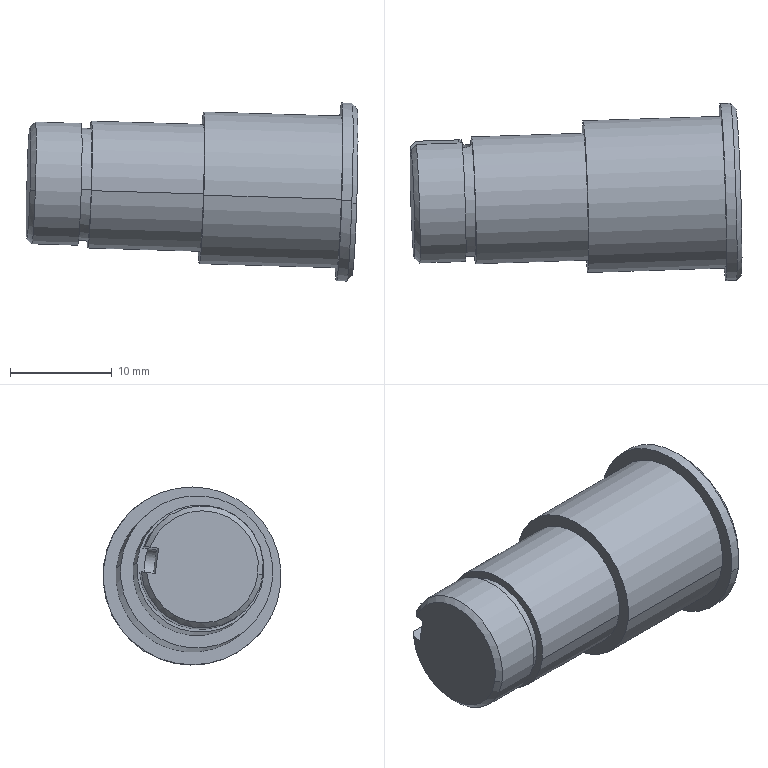Part | STEP file | 2026.6.15-Main Assembly图.sldasm-Part-130 | 1 solid | 24 faces | box 32.571 x 17.473 x 17.472 mm | volume 4708 mm3 | cylinder 11 | plane 9 | cone 4 | commonest cylinder face diameters 11 x3 12.5 x2 14.95 x2 17.45 x2 2.5 x1 12 x1
STEP:
#1=CARTESIAN_POINT('',(-1558.702,1426.585,3693.659));
#2=VERTEX_POINT('',#1);
#3=CARTESIAN_POINT('',(-1558.329,1414.148,3692.46));
#4=VERTEX_POINT('',#3);
#5=CARTESIAN_POINT('',(-1558.516,1420.367,3693.06));
#6=DIRECTION('',(-0.999,-0.03277,0.02917));
#7=DIRECTION('',(-0.02983,0.9949,0.09589));
#8=AXIS2_PLACEMENT_3D('',#5,#6,#7);
#9=CIRCLE('',#8,6.25);
#10=EDGE_CURVE('',#2,#4,#9,.T.);
#11=ORIENTED_EDGE('',*,*,#10,.T.);
#12=CARTESIAN_POINT('',(-1569.319,1413.788,3692.781));
#13=VERTEX_POINT('',#12);
#14=CARTESIAN_POINT('',(-1558.329,1414.148,3692.46));
#15=DIRECTION('',(-0.999,-0.03277,0.02917));
#16=VECTOR('',#15,1000.);
#17=LINE('',#14,#16);
#18=EDGE_CURVE('',#4,#13,#17,.T.);
#19=ORIENTED_EDGE('',*,*,#18,.T.);
#20=CARTESIAN_POINT('',(-1569.692,1426.225,3693.98));
#21=VERTEX_POINT('',#20);
#22=CARTESIAN_POINT('',(-1569.505,1420.006,3693.381));
#23=DIRECTION('',(0.999,0.03277,-0.02917));
#24=DIRECTION('',(-0.02983,0.9949,0.09589));
#25=AXIS2_PLACEMENT_3D('',#22,#23,#24);
#26=CIRCLE('',#25,6.25);
#27=EDGE_CURVE('',#13,#21,#26,.T.);
#28=ORIENTED_EDGE('',*,*,#27,.T.);
#29=CARTESIAN_POINT('',(-1558.702,1426.585,3693.659));
#30=DIRECTION('',(-0.999,-0.03277,0.02917));
#31=VECTOR('',#30,1000.);
#32=LINE('',#29,#31);
#33=EDGE_CURVE('',#2,#21,#32,.T.);
#34=ORIENTED_EDGE('',*,*,#33,.F.);
#35=EDGE_LOOP('',(#11,#19,#28,#34));
#36=FACE_OUTER_BOUND('',#35,.T.);
#37=CARTESIAN_POINT('',(-1558.516,1420.367,3693.06));
#38=DIRECTION('',(-0.999,-0.03277,0.02917));
#39=DIRECTION('',(-0.02983,0.9949,0.09589));
#40=AXIS2_PLACEMENT_3D('',#37,#38,#39);
#41=CYLINDRICAL_SURFACE('',#40,6.25);
#42=ADVANCED_FACE('',(#36),#41,.T.);
#43=CARTESIAN_POINT('',(-1545.252,1428.246,3693.383));
#44=VERTEX_POINT('',#43);
#45=CARTESIAN_POINT('',(-1544.806,1413.372,3691.949));
#46=VERTEX_POINT('',#45);
#47=CARTESIAN_POINT('',(-1545.029,1420.809,3692.666));
#48=DIRECTION('',(-0.999,-0.03277,0.02917));
#49=DIRECTION('',(-0.02983,0.9949,0.09589));
#50=AXIS2_PLACEMENT_3D('',#47,#48,#49);
#51=CIRCLE('',#50,7.475);
#52=EDGE_CURVE('',#44,#46,#51,.T.);
#53=ORIENTED_EDGE('',*,*,#52,.T.);
#54=CARTESIAN_POINT('',(-1558.293,1412.929,3692.343));
#55=VERTEX_POINT('',#54);
#56=CARTESIAN_POINT('',(-1544.806,1413.372,3691.949));
#57=DIRECTION('',(-0.999,-0.03277,0.02917));
#58=VECTOR('',#57,1000.);
#59=LINE('',#56,#58);
#60=EDGE_CURVE('',#46,#55,#59,.T.);
#61=ORIENTED_EDGE('',*,*,#60,.T.);
#62=CARTESIAN_POINT('',(-1558.739,1427.804,3693.776));
#63=VERTEX_POINT('',#62);
#64=CARTESIAN_POINT('',(-1558.516,1420.367,3693.06));
#65=DIRECTION('',(0.999,0.03277,-0.02917));
#66=DIRECTION('',(-0.02983,0.9949,0.09589));
#67=AXIS2_PLACEMENT_3D('',#64,#65,#66);
#68=CIRCLE('',#67,7.475);
#69=EDGE_CURVE('',#55,#63,#68,.T.);
#70=ORIENTED_EDGE('',*,*,#69,.T.);
#71=CARTESIAN_POINT('',(-1545.252,1428.246,3693.383));
#72=DIRECTION('',(-0.999,-0.03277,0.02917));
#73=VECTOR('',#72,1000.);
#74=LINE('',#71,#73);
#75=EDGE_CURVE('',#44,#63,#74,.T.);
#76=ORIENTED_EDGE('',*,*,#75,.F.);
#77=EDGE_LOOP('',(#53,#61,#70,#76));
#78=FACE_OUTER_BOUND('',#77,.T.);
#79=CARTESIAN_POINT('',(-1545.029,1420.809,3692.666));
#80=DIRECTION('',(-0.999,-0.03277,0.02917));
#81=DIRECTION('',(-0.02983,0.9949,0.09589));
#82=AXIS2_PLACEMENT_3D('',#79,#80,#81);
#83=CYLINDRICAL_SURFACE('',#82,7.475);
#84=ADVANCED_FACE('',(#78),#83,.T.);
#85=CARTESIAN_POINT('',(-1543.294,1412.706,3691.557));
#86=VERTEX_POINT('',#85);
#87=CARTESIAN_POINT('',(-1543.767,1429.01,3693.687));
#88=VERTEX_POINT('',#87);
#89=CARTESIAN_POINT('',(-1543.53,1420.858,3692.622));
#90=DIRECTION('',(0.999,0.03277,-0.02917));
#91=DIRECTION('',(0.02873,-0.9912,-0.1295));
#92=AXIS2_PLACEMENT_3D('',#89,#90,#91);
#93=CIRCLE('',#92,8.225);
#94=EDGE_CURVE('',#86,#88,#93,.T.);
#95=ORIENTED_EDGE('',*,*,#94,.F.);
#96=CARTESIAN_POINT('',(-1543.779,1412.194,3691.507));
#97=VERTEX_POINT('',#96);
#98=CARTESIAN_POINT('',(-1543.779,1412.194,3691.507));
#99=DIRECTION('',(-0.6861,-0.724,-0.07092));
#100=VECTOR('',#99,1000.);
#101=LINE('',#98,#100);
#102=EDGE_CURVE('',#86,#97,#101,.T.);
#103=ORIENTED_EDGE('',*,*,#102,.T.);
#104=CARTESIAN_POINT('',(-1544.29,1429.523,3693.473));
#105=VERTEX_POINT('',#104);
#106=CARTESIAN_POINT('',(-1544.03,1420.842,3692.637));
#107=DIRECTION('',(-0.999,-0.03277,0.02917));
#108=DIRECTION('',(0.02873,-0.9912,-0.1295));
#109=AXIS2_PLACEMENT_3D('',#106,#107,#108);
#110=CIRCLE('',#109,8.725);
#111=EDGE_CURVE('',#105,#97,#110,.T.);
#112=ORIENTED_EDGE('',*,*,#111,.F.);
#113=CARTESIAN_POINT('',(-1544.281,1429.49,3693.766));
#114=VERTEX_POINT('',#113);
#115=CARTESIAN_POINT('',(-1544.03,1420.842,3692.637));
#116=DIRECTION('',(-0.999,-0.03277,0.02917));
#117=DIRECTION('',(0.02873,-0.9912,-0.1295));
#118=AXIS2_PLACEMENT_3D('',#115,#116,#117);
#119=CIRCLE('',#118,8.725);
#120=EDGE_CURVE('',#114,#105,#119,.T.);
#121=ORIENTED_EDGE('',*,*,#120,.F.);
#122=CARTESIAN_POINT('',(-1544.281,1429.49,3693.766));
#123=DIRECTION('',(-0.7267,0.6777,0.1122));
#124=VECTOR('',#123,1000.);
#125=LINE('',#122,#124);
#126=EDGE_CURVE('',#88,#114,#125,.T.);
#127=ORIENTED_EDGE('',*,*,#126,.F.);
#128=EDGE_LOOP('',(#95,#103,#112,#121,#127));
#129=FACE_OUTER_BOUND('',#128,.T.);
#130=CARTESIAN_POINT('',(-1544.03,1420.842,3692.637));
#131=DIRECTION('',(-0.999,-0.03277,0.02917));
#132=DIRECTION('',(-0.02873,0.9912,0.1295));
#133=AXIS2_PLACEMENT_3D('',#130,#131,#132);
#134=CONICAL_SURFACE('',#133,8.725,0.7854);
#135=ADVANCED_FACE('',(#129),#134,.T.);
#136=ORIENTED_EDGE('',*,*,#111,.T.);
#137=CARTESIAN_POINT('',(-1543.77,1412.161,3691.8));
#138=VERTEX_POINT('',#137);
#139=CARTESIAN_POINT('',(-1544.03,1420.842,3692.637));
#140=DIRECTION('',(-0.999,-0.03277,0.02917));
#141=DIRECTION('',(0.02873,-0.9912,-0.1295));
#142=AXIS2_PLACEMENT_3D('',#139,#140,#141);
#143=CIRCLE('',#142,8.725);
#144=EDGE_CURVE('',#97,#138,#143,.T.);
#145=ORIENTED_EDGE('',*,*,#144,.T.);
#146=CARTESIAN_POINT('',(-1544.769,1412.128,3691.829));
#147=VERTEX_POINT('',#146);
#148=CARTESIAN_POINT('',(-1543.27,1412.177,3691.785));
#149=DIRECTION('',(-0.999,-0.03277,0.02917));
#150=VECTOR('',#149,1000.);
#151=LINE('',#148,#150);
#152=EDGE_CURVE('',#138,#147,#151,.T.);
#153=ORIENTED_EDGE('',*,*,#152,.T.);
#154=CARTESIAN_POINT('',(-1545.289,1429.49,3693.502));
#155=VERTEX_POINT('',#154);
#156=CARTESIAN_POINT('',(-1545.029,1420.809,3692.666));
#157=DIRECTION('',(0.999,0.03277,-0.02917));
#158=DIRECTION('',(-0.02983,0.9949,0.09589));
#159=AXIS2_PLACEMENT_3D('',#156,#157,#158);
#160=CIRCLE('',#159,8.725);
#161=EDGE_CURVE('',#147,#155,#160,.T.);
#162=ORIENTED_EDGE('',*,*,#161,.T.);
#163=CARTESIAN_POINT('',(-1543.791,1429.539,3693.459));
#164=DIRECTION('',(-0.999,-0.03277,0.02917));
#165=VECTOR('',#164,1000.);
#166=LINE('',#163,#165);
#167=EDGE_CURVE('',#105,#155,#166,.T.);
#168=ORIENTED_EDGE('',*,*,#167,.F.);
#169=EDGE_LOOP('',(#136,#145,#153,#162,#168));
#170=FACE_OUTER_BOUND('',#169,.T.);
#171=CARTESIAN_POINT('',(-1543.53,1420.858,3692.622));
#172=DIRECTION('',(-0.999,-0.03277,0.02917));
#173=DIRECTION('',(-0.02983,0.9949,0.09589));
#174=AXIS2_PLACEMENT_3D('',#171,#172,#173);
#175=CYLINDRICAL_SURFACE('',#174,8.725);
#176=ADVANCED_FACE('',(#170),#175,.T.);
#177=CARTESIAN_POINT('',(-1575.342,1414.358,3692.843));
#178=VERTEX_POINT('',#177);
#179=CARTESIAN_POINT('',(-1575.612,1424.958,3695.488));
#180=VERTEX_POINT('',#179);
#181=CARTESIAN_POINT('',(-1575.5,1419.809,3693.556));
#182=DIRECTION('',(-0.999,-0.03277,0.02917));
#183=DIRECTION('',(-0.02873,0.9912,0.1295));
#184=AXIS2_PLACEMENT_3D('',#181,#182,#183);
#185=CIRCLE('',#184,5.5);
#186=EDGE_CURVE('',#178,#180,#185,.T.);
#187=ORIENTED_EDGE('',*,*,#186,.F.);
#188=CARTESIAN_POINT('',(-1574.828,1413.879,3692.764));
#189=VERTEX_POINT('',#188);
#190=CARTESIAN_POINT('',(-1574.828,1413.879,3692.764));
#191=DIRECTION('',(0.7267,-0.6777,-0.1122));
#192=VECTOR('',#191,1000.);
#193=LINE('',#190,#192);
#194=EDGE_CURVE('',#178,#189,#193,.T.);
#195=ORIENTED_EDGE('',*,*,#194,.T.);
#196=CARTESIAN_POINT('',(-1575.127,1425.482,3695.54));
#197=VERTEX_POINT('',#196);
#198=CARTESIAN_POINT('',(-1575.,1419.826,3693.541));
#199=DIRECTION('',(0.999,0.03277,-0.02917));
#200=DIRECTION('',(-0.02873,0.9912,0.1295));
#201=AXIS2_PLACEMENT_3D('',#198,#199,#200);
#202=CIRCLE('',#201,6.);
#203=EDGE_CURVE('',#197,#189,#202,.T.);
#204=ORIENTED_EDGE('',*,*,#203,.F.);
#205=CARTESIAN_POINT('',(-1575.127,1425.482,3695.54));
#206=CARTESIAN_POINT('',(-1575.289,1425.307,3695.523));
#207=CARTESIAN_POINT('',(-1575.451,1425.132,3695.505));
#208=CARTESIAN_POINT('',(-1575.612,1424.958,3695.488));
#209=B_SPLINE_CURVE_WITH_KNOTS('',3,(#205,#206,#207,#208),.UNSPECIFIED.,.F.,.F.,(4,4),(0.002943,0.003659),.UNSPECIFIED.);
#210=EDGE_CURVE('',#197,#180,#209,.T.);
#211=ORIENTED_EDGE('',*,*,#210,.T.);
#212=EDGE_LOOP('',(#187,#195,#204,#211));
#213=FACE_OUTER_BOUND('',#212,.T.);
#214=CARTESIAN_POINT('',(-1575.,1419.826,3693.541));
#215=DIRECTION('',(0.999,0.03277,-0.02917));
#216=DIRECTION('',(0.02873,-0.9912,-0.1295));
#217=AXIS2_PLACEMENT_3D('',#214,#215,#216);
#218=CONICAL_SURFACE('',#217,6.,0.7854);
#219=ADVANCED_FACE('',(#213),#218,.T.);
#220=CARTESIAN_POINT('',(-1569.669,1425.478,3693.908));
#221=VERTEX_POINT('',#220);
#222=CARTESIAN_POINT('',(-1569.341,1414.534,3692.853));
#223=VERTEX_POINT('',#222);
#224=CARTESIAN_POINT('',(-1569.505,1420.006,3693.381));
#225=DIRECTION('',(-0.999,-0.03277,0.02917));
#226=DIRECTION('',(-0.02983,0.9949,0.09589));
#227=AXIS2_PLACEMENT_3D('',#224,#225,#226);
#228=CIRCLE('',#227,5.5);
#229=EDGE_CURVE('',#221,#223,#228,.T.);
#230=ORIENTED_EDGE('',*,*,#229,.T.);
#231=CARTESIAN_POINT('',(-1570.34,1414.501,3692.882));
#232=VERTEX_POINT('',#231);
#233=CARTESIAN_POINT('',(-1569.341,1414.534,3692.853));
#234=DIRECTION('',(-0.999,-0.03277,0.02917));
#235=VECTOR('',#234,1000.);
#236=LINE('',#233,#235);
#237=EDGE_CURVE('',#223,#232,#236,.T.);
#238=ORIENTED_EDGE('',*,*,#237,.T.);
#239=CARTESIAN_POINT('',(-1570.699,1425.445,3692.89));
#240=VERTEX_POINT('',#239);
#241=CARTESIAN_POINT('',(-1570.504,1419.973,3693.41));
#242=DIRECTION('',(0.999,0.03277,-0.02917));
#243=DIRECTION('',(-0.02983,0.9949,0.09589));
#244=AXIS2_PLACEMENT_3D('',#241,#242,#243);
#245=CIRCLE('',#244,5.5);
#246=EDGE_CURVE('',#232,#240,#245,.T.);
#247=ORIENTED_EDGE('',*,*,#246,.T.);
#248=CARTESIAN_POINT('',(-1569.683,1425.478,3693.908));
#249=VERTEX_POINT('',#248);
#250=CARTESIAN_POINT('',(-1570.699,1425.445,3692.89));
#251=CARTESIAN_POINT('',(-1570.572,1425.452,3692.913));
#252=CARTESIAN_POINT('',(-1570.452,1425.46,3692.954));
#253=CARTESIAN_POINT('',(-1570.226,1425.476,3693.074));
#254=CARTESIAN_POINT('',(-1570.123,1425.484,3693.15));
#255=CARTESIAN_POINT('',(-1569.853,1425.501,3693.422));
#256=CARTESIAN_POINT('',(-1569.729,1425.5,3693.66));
#257=CARTESIAN_POINT('',(-1569.683,1425.478,3693.908));
#258=B_SPLINE_CURVE_WITH_KNOTS('',3,(#250,#251,#252,#253,#254,#255,#256,#257),.UNSPECIFIED.,.F.,.F.,(4,2,2,4),(0.,0.0003812,0.0007624,0.001525),.UNSPECIFIED.);
#259=EDGE_CURVE('',#240,#249,#258,.T.);
#260=ORIENTED_EDGE('',*,*,#259,.T.);
#261=CARTESIAN_POINT('',(-1569.669,1425.478,3693.908));
#262=DIRECTION('',(-0.999,-0.03277,0.02917));
#263=VECTOR('',#262,1000.);
#264=LINE('',#261,#263);
#265=EDGE_CURVE('',#221,#249,#264,.T.);
#266=ORIENTED_EDGE('',*,*,#265,.F.);
#267=EDGE_LOOP('',(#230,#238,#247,#260,#266));
#268=FACE_OUTER_BOUND('',#267,.T.);
#269=CARTESIAN_POINT('',(-1569.505,1420.006,3693.381));
#270=DIRECTION('',(-0.999,-0.03277,0.02917));
#271=DIRECTION('',(-0.02983,0.9949,0.09589));
#272=AXIS2_PLACEMENT_3D('',#269,#270,#271);
#273=CYLINDRICAL_SURFACE('',#272,5.5);
#274=ADVANCED_FACE('',(#268),#273,.T.);
#275=CARTESIAN_POINT('',(-1569.663,1425.458,3694.093));
#276=VERTEX_POINT('',#275);
#277=CARTESIAN_POINT('',(-1569.505,1420.006,3693.381));
#278=DIRECTION('',(-0.999,-0.03277,0.02917));
#279=DIRECTION('',(-0.02983,0.9949,0.09589));
#280=AXIS2_PLACEMENT_3D('',#277,#278,#279);
#281=CIRCLE('',#280,5.5);
#282=EDGE_CURVE('',#276,#221,#281,.T.);
#283=ORIENTED_EDGE('',*,*,#282,.T.);
#284=ORIENTED_EDGE('',*,*,#265,.T.);
#285=CARTESIAN_POINT('',(-1569.683,1425.478,3693.908));
#286=CARTESIAN_POINT('',(-1569.672,1425.472,3693.969));
#287=CARTESIAN_POINT('',(-1569.665,1425.466,3694.03));
#288=CARTESIAN_POINT('',(-1569.663,1425.458,3694.093));
#289=B_SPLINE_CURVE_WITH_KNOTS('',3,(#285,#286,#287,#288),.UNSPECIFIED.,.F.,.F.,(4,4),(0.001525,0.001711),.UNSPECIFIED.);
#290=EDGE_CURVE('',#249,#276,#289,.T.);
#291=ORIENTED_EDGE('',*,*,#290,.T.);
#292=EDGE_LOOP('',(#283,#284,#291));
#293=FACE_OUTER_BOUND('',#292,.T.);
#294=CARTESIAN_POINT('',(-1569.505,1420.006,3693.381));
#295=DIRECTION('',(-0.999,-0.03277,0.02917));
#296=DIRECTION('',(-0.02983,0.9949,0.09589));
#297=AXIS2_PLACEMENT_3D('',#294,#295,#296);
#298=CYLINDRICAL_SURFACE('',#297,5.5);
#299=ADVANCED_FACE('',(#293),#298,.T.);
#300=ORIENTED_EDGE('',*,*,#237,.F.);
#301=CARTESIAN_POINT('',(-1569.505,1420.006,3693.381));
#302=DIRECTION('',(-0.999,-0.03277,0.02917));
#303=DIRECTION('',(-0.02983,0.9949,0.09589));
#304=AXIS2_PLACEMENT_3D('',#301,#302,#303);
#305=CIRCLE('',#304,5.5);
#306=EDGE_CURVE('',#223,#276,#305,.T.);
#307=ORIENTED_EDGE('',*,*,#306,.T.);
#308=CARTESIAN_POINT('',(-1570.618,1425.13,3695.318));
#309=VERTEX_POINT('',#308);
#310=CARTESIAN_POINT('',(-1569.663,1425.458,3694.093));
#311=CARTESIAN_POINT('',(-1569.659,1425.439,3694.236));
#312=CARTESIAN_POINT('',(-1569.678,1425.414,3694.376));
#313=CARTESIAN_POINT('',(-1569.766,1425.356,3694.645));
#314=CARTESIAN_POINT('',(-1569.831,1425.323,3694.768));
#315=CARTESIAN_POINT('',(-1570.004,1425.257,3694.989));
#316=CARTESIAN_POINT('',(-1570.109,1425.224,3695.082));
#317=CARTESIAN_POINT('',(-1570.348,1425.168,3695.232));
#318=CARTESIAN_POINT('',(-1570.478,1425.145,3695.286));
#319=CARTESIAN_POINT('',(-1570.618,1425.13,3695.318));
#320=B_SPLINE_CURVE_WITH_KNOTS('',3,(#310,#311,#312,#313,#314,#315,#316,#317,#318,#319),.UNSPECIFIED.,.F.,.F.,(4,2,2,2,4),(0.,0.0004277,0.0008554,0.001283,0.001711),.UNSPECIFIED.);
#321=EDGE_CURVE('',#276,#309,#320,.T.);
#322=ORIENTED_EDGE('',*,*,#321,.T.);
#323=CARTESIAN_POINT('',(-1570.504,1419.973,3693.41));
#324=DIRECTION('',(0.999,0.03277,-0.02917));
#325=DIRECTION('',(-0.02983,0.9949,0.09589));
#326=AXIS2_PLACEMENT_3D('',#323,#324,#325);
#327=CIRCLE('',#326,5.5);
#328=EDGE_CURVE('',#309,#232,#327,.T.);
#329=ORIENTED_EDGE('',*,*,#328,.T.);
#330=EDGE_LOOP('',(#300,#307,#322,#329));
#331=FACE_OUTER_BOUND('',#330,.T.);
#332=CARTESIAN_POINT('',(-1569.505,1420.006,3693.381));
#333=DIRECTION('',(-0.999,-0.03277,0.02917));
#334=DIRECTION('',(-0.02983,0.9949,0.09589));
#335=AXIS2_PLACEMENT_3D('',#332,#333,#334);
#336=CYLINDRICAL_SURFACE('',#335,5.5);
#337=ADVANCED_FACE('',(#331),#336,.T.);
#338=ORIENTED_EDGE('',*,*,#328,.F.);
#339=CARTESIAN_POINT('',(-1570.633,1425.638,3695.384));
#340=VERTEX_POINT('',#339);
#341=CARTESIAN_POINT('',(-1570.618,1425.13,3695.318));
#342=DIRECTION('',(-0.02873,0.9912,0.1295));
#343=VECTOR('',#342,1000.);
#344=LINE('',#341,#343);
#345=EDGE_CURVE('',#309,#340,#344,.T.);
#346=ORIENTED_EDGE('',*,*,#345,.T.);
#347=CARTESIAN_POINT('',(-1570.714,1425.953,3692.956));
#348=VERTEX_POINT('',#347);
#349=CARTESIAN_POINT('',(-1570.504,1419.973,3693.41));
#350=DIRECTION('',(-0.999,-0.03277,0.02917));
#351=DIRECTION('',(-0.02983,0.9949,0.09589));
#352=AXIS2_PLACEMENT_3D('',#349,#350,#351);
#353=CIRCLE('',#352,6.);
#354=EDGE_CURVE('',#348,#340,#353,.T.);
#355=ORIENTED_EDGE('',*,*,#354,.F.);
#356=CARTESIAN_POINT('',(-1570.714,1425.953,3692.956));
#357=DIRECTION('',(0.02873,-0.9912,-0.1295));
#358=VECTOR('',#357,1000.);
#359=LINE('',#356,#358);
#360=EDGE_CURVE('',#348,#240,#359,.T.);
#361=ORIENTED_EDGE('',*,*,#360,.T.);
#362=ORIENTED_EDGE('',*,*,#246,.F.);
#363=EDGE_LOOP('',(#338,#346,#355,#361,#362));
#364=FACE_OUTER_BOUND('',#363,.T.);
#365=CARTESIAN_POINT('',(-1570.504,1419.973,3693.41));
#366=DIRECTION('',(0.999,0.03277,-0.02917));
#367=DIRECTION('',(0.02873,-0.9912,-0.1295));
#368=AXIS2_PLACEMENT_3D('',#365,#366,#367);
#369=PLANE('',#368);
#370=ADVANCED_FACE('',(#364),#369,.T.);
#371=ORIENTED_EDGE('',*,*,#354,.T.);
#372=CARTESIAN_POINT('',(-1570.881,1425.621,3695.416));
#373=VERTEX_POINT('',#372);
#374=CARTESIAN_POINT('',(-1570.633,1425.638,3695.384));
#375=CARTESIAN_POINT('',(-1570.714,1425.629,3695.403));
#376=CARTESIAN_POINT('',(-1570.797,1425.624,3695.413));
#377=CARTESIAN_POINT('',(-1570.881,1425.621,3695.416));
#378=B_SPLINE_CURVE_WITH_KNOTS('',3,(#374,#375,#376,#377),.UNSPECIFIED.,.F.,.F.,(4,4),(0.,0.0002513),.UNSPECIFIED.);
#379=EDGE_CURVE('',#340,#373,#378,.T.);
#380=ORIENTED_EDGE('',*,*,#379,.T.);
#381=CARTESIAN_POINT('',(-1570.632,1425.629,3695.408));
#382=DIRECTION('',(-0.999,-0.03277,0.02917));
#383=VECTOR('',#382,1000.);
#384=LINE('',#381,#383);
#385=EDGE_CURVE('',#373,#197,#384,.T.);
#386=ORIENTED_EDGE('',*,*,#385,.T.);
#387=ORIENTED_EDGE('',*,*,#203,.T.);
#388=CARTESIAN_POINT('',(-1575.21,1425.803,3693.062));
#389=VERTEX_POINT('',#388);
#390=CARTESIAN_POINT('',(-1575.,1419.826,3693.541));
#391=DIRECTION('',(0.999,0.03277,-0.02917));
#392=DIRECTION('',(-0.02873,0.9912,0.1295));
#393=AXIS2_PLACEMENT_3D('',#390,#391,#392);
#394=CIRCLE('',#393,6.);
#395=EDGE_CURVE('',#189,#389,#394,.T.);
#396=ORIENTED_EDGE('',*,*,#395,.T.);
#397=CARTESIAN_POINT('',(-1570.964,1425.942,3692.938));
#398=VERTEX_POINT('',#397);
#399=CARTESIAN_POINT('',(-1570.714,1425.95,3692.931));
#400=DIRECTION('',(-0.999,-0.03277,0.02917));
#401=VECTOR('',#400,1000.);
#402=LINE('',#399,#401);
#403=EDGE_CURVE('',#398,#389,#402,.T.);
#404=ORIENTED_EDGE('',*,*,#403,.F.);
#405=CARTESIAN_POINT('',(-1570.964,1425.942,3692.938));
#406=CARTESIAN_POINT('',(-1570.88,1425.945,3692.935));
#407=CARTESIAN_POINT('',(-1570.797,1425.948,3692.942));
#408=CARTESIAN_POINT('',(-1570.714,1425.953,3692.956));
#409=B_SPLINE_CURVE_WITH_KNOTS('',3,(#405,#406,#407,#408),.UNSPECIFIED.,.F.,.F.,(4,4),(0.,0.0002513),.UNSPECIFIED.);
#410=EDGE_CURVE('',#398,#348,#409,.T.);
#411=ORIENTED_EDGE('',*,*,#410,.T.);
#412=EDGE_LOOP('',(#371,#380,#386,#387,#396,#404,#411));
#413=FACE_OUTER_BOUND('',#412,.T.);
#414=CARTESIAN_POINT('',(-1570.504,1419.973,3693.41));
#415=DIRECTION('',(-0.999,-0.03277,0.02917));
#416=DIRECTION('',(-0.02983,0.9949,0.09589));
#417=AXIS2_PLACEMENT_3D('',#414,#415,#416);
#418=CYLINDRICAL_SURFACE('',#417,6.);
#419=ADVANCED_FACE('',(#413),#418,.T.);
#420=ORIENTED_EDGE('',*,*,#194,.F.);
#421=CARTESIAN_POINT('',(-1575.695,1425.279,3693.01));
#422=VERTEX_POINT('',#421);
#423=CARTESIAN_POINT('',(-1575.5,1419.809,3693.556));
#424=DIRECTION('',(-0.999,-0.03277,0.02917));
#425=DIRECTION('',(-0.02873,0.9912,0.1295));
#426=AXIS2_PLACEMENT_3D('',#423,#424,#425);
#427=CIRCLE('',#426,5.5);
#428=EDGE_CURVE('',#422,#178,#427,.T.);
#429=ORIENTED_EDGE('',*,*,#428,.F.);
#430=CARTESIAN_POINT('',(-1575.21,1425.803,3693.062));
#431=CARTESIAN_POINT('',(-1575.372,1425.628,3693.045));
#432=CARTESIAN_POINT('',(-1575.534,1425.454,3693.027));
#433=CARTESIAN_POINT('',(-1575.695,1425.279,3693.01));
#434=B_SPLINE_CURVE_WITH_KNOTS('',3,(#430,#431,#432,#433),.UNSPECIFIED.,.F.,.F.,(4,4),(0.002943,0.003659),.UNSPECIFIED.);
#435=EDGE_CURVE('',#389,#422,#434,.T.);
#436=ORIENTED_EDGE('',*,*,#435,.F.);
#437=ORIENTED_EDGE('',*,*,#395,.F.);
#438=EDGE_LOOP('',(#420,#429,#436,#437));
#439=FACE_OUTER_BOUND('',#438,.T.);
#440=CARTESIAN_POINT('',(-1575.,1419.826,3693.541));
#441=DIRECTION('',(0.999,0.03277,-0.02917));
#442=DIRECTION('',(0.02873,-0.9912,-0.1295));
#443=AXIS2_PLACEMENT_3D('',#440,#441,#442);
#444=CONICAL_SURFACE('',#443,6.,0.7854);
#445=ADVANCED_FACE('',(#439),#444,.T.);
#446=ORIENTED_EDGE('',*,*,#52,.F.);
#447=CARTESIAN_POINT('',(-1545.029,1420.809,3692.666));
#448=DIRECTION('',(-0.999,-0.03277,0.02917));
#449=DIRECTION('',(-0.02983,0.9949,0.09589));
#450=AXIS2_PLACEMENT_3D('',#447,#448,#449);
#451=CIRCLE('',#450,7.475);
#452=EDGE_CURVE('',#46,#44,#451,.T.);
#453=ORIENTED_EDGE('',*,*,#452,.F.);
#454=EDGE_LOOP('',(#446,#453));
#455=FACE_BOUND('',#454,.T.);
#456=CARTESIAN_POINT('',(-1545.029,1420.809,3692.666));
#457=DIRECTION('',(0.999,0.03277,-0.02917));
#458=DIRECTION('',(-0.02983,0.9949,0.09589));
#459=AXIS2_PLACEMENT_3D('',#456,#457,#458);
#460=CIRCLE('',#459,8.725);
#461=EDGE_CURVE('',#155,#147,#460,.T.);
#462=ORIENTED_EDGE('',*,*,#461,.F.);
#463=ORIENTED_EDGE('',*,*,#161,.F.);
#464=EDGE_LOOP('',(#462,#463));
#465=FACE_OUTER_BOUND('',#464,.T.);
#466=CARTESIAN_POINT('',(-1545.029,1420.809,3692.666));
#467=DIRECTION('',(-0.999,-0.03277,0.02917));
#468=DIRECTION('',(-0.02873,0.9912,0.1295));
#469=AXIS2_PLACEMENT_3D('',#466,#467,#468);
#470=PLANE('',#469);
#471=ADVANCED_FACE('',(#455,#465),#470,.T.);
#472=CARTESIAN_POINT('',(-1543.53,1420.858,3692.622));
#473=DIRECTION('',(0.999,0.03277,-0.02917));
#474=DIRECTION('',(0.02873,-0.9912,-0.1295));
#475=AXIS2_PLACEMENT_3D('',#472,#473,#474);
#476=CIRCLE('',#475,8.225);
#477=EDGE_CURVE('',#88,#86,#476,.T.);
#478=ORIENTED_EDGE('',*,*,#477,.T.);
#479=ORIENTED_EDGE('',*,*,#94,.T.);
#480=EDGE_LOOP('',(#478,#479));
#481=FACE_OUTER_BOUND('',#480,.T.);
#482=CARTESIAN_POINT('',(-1543.53,1420.858,3692.622));
#483=DIRECTION('',(0.999,0.03277,-0.02917));
#484=DIRECTION('',(0.02873,-0.9912,-0.1295));
#485=AXIS2_PLACEMENT_3D('',#482,#483,#484);
#486=PLANE('',#485);
#487=ADVANCED_FACE('',(#481),#486,.T.);
#488=ORIENTED_EDGE('',*,*,#152,.F.);
#489=CARTESIAN_POINT('',(-1544.03,1420.842,3692.637));
#490=DIRECTION('',(-0.999,-0.03277,0.02917));
#491=DIRECTION('',(0.02873,-0.9912,-0.1295));
#492=AXIS2_PLACEMENT_3D('',#489,#490,#491);
#493=CIRCLE('',#492,8.725);
#494=EDGE_CURVE('',#138,#114,#493,.T.);
#495=ORIENTED_EDGE('',*,*,#494,.T.);
#496=ORIENTED_EDGE('',*,*,#120,.T.);
#497=ORIENTED_EDGE('',*,*,#167,.T.);
#498=ORIENTED_EDGE('',*,*,#461,.T.);
#499=EDGE_LOOP('',(#488,#495,#496,#497,#498));
#500=FACE_OUTER_BOUND('',#499,.T.);
#501=CARTESIAN_POINT('',(-1543.53,1420.858,3692.622));
#502=DIRECTION('',(-0.999,-0.03277,0.02917));
#503=DIRECTION('',(-0.02983,0.9949,0.09589));
#504=AXIS2_PLACEMENT_3D('',#501,#502,#503);
#505=CYLINDRICAL_SURFACE('',#504,8.725);
#506=ADVANCED_FACE('',(#500),#505,.T.);
#507=ORIENTED_EDGE('',*,*,#102,.F.);
#508=ORIENTED_EDGE('',*,*,#477,.F.);
#509=ORIENTED_EDGE('',*,*,#126,.T.);
#510=ORIENTED_EDGE('',*,*,#494,.F.);
#511=ORIENTED_EDGE('',*,*,#144,.F.);
#512=EDGE_LOOP('',(#507,#508,#509,#510,#511));
#513=FACE_OUTER_BOUND('',#512,.T.);
#514=CARTESIAN_POINT('',(-1544.03,1420.842,3692.637));
#515=DIRECTION('',(-0.999,-0.03277,0.02917));
#516=DIRECTION('',(-0.02873,0.9912,0.1295));
#517=AXIS2_PLACEMENT_3D('',#514,#515,#516);
#518=CONICAL_SURFACE('',#517,8.725,0.7854);
#519=ADVANCED_FACE('',(#513),#518,.T.);
#520=ORIENTED_EDGE('',*,*,#10,.F.);
#521=CARTESIAN_POINT('',(-1558.516,1420.367,3693.06));
#522=DIRECTION('',(-0.999,-0.03277,0.02917));
#523=DIRECTION('',(-0.02983,0.9949,0.09589));
#524=AXIS2_PLACEMENT_3D('',#521,#522,#523);
#525=CIRCLE('',#524,6.25);
#526=EDGE_CURVE('',#4,#2,#525,.T.);
#527=ORIENTED_EDGE('',*,*,#526,.F.);
#528=EDGE_LOOP('',(#520,#527));
#529=FACE_BOUND('',#528,.T.);
#530=CARTESIAN_POINT('',(-1558.516,1420.367,3693.06));
#531=DIRECTION('',(0.999,0.03277,-0.02917));
#532=DIRECTION('',(-0.02983,0.9949,0.09589));
#533=AXIS2_PLACEMENT_3D('',#530,#531,#532);
#534=CIRCLE('',#533,7.475);
#535=EDGE_CURVE('',#63,#55,#534,.T.);
#536=ORIENTED_EDGE('',*,*,#535,.F.);
#537=ORIENTED_EDGE('',*,*,#69,.F.);
#538=EDGE_LOOP('',(#536,#537));
#539=FACE_OUTER_BOUND('',#538,.T.);
#540=CARTESIAN_POINT('',(-1558.516,1420.367,3693.06));
#541=DIRECTION('',(-0.999,-0.03277,0.02917));
#542=DIRECTION('',(-0.02873,0.9912,0.1295));
#543=AXIS2_PLACEMENT_3D('',#540,#541,#542);
#544=PLANE('',#543);
#545=ADVANCED_FACE('',(#529,#539),#544,.T.);
#546=ORIENTED_EDGE('',*,*,#60,.F.);
#547=ORIENTED_EDGE('',*,*,#452,.T.);
#548=ORIENTED_EDGE('',*,*,#75,.T.);
#549=ORIENTED_EDGE('',*,*,#535,.T.);
#550=EDGE_LOOP('',(#546,#547,#548,#549));
#551=FACE_OUTER_BOUND('',#550,.T.);
#552=CARTESIAN_POINT('',(-1545.029,1420.809,3692.666));
#553=DIRECTION('',(-0.999,-0.03277,0.02917));
#554=DIRECTION('',(-0.02983,0.9949,0.09589));
#555=AXIS2_PLACEMENT_3D('',#552,#553,#554);
#556=CYLINDRICAL_SURFACE('',#555,7.475);
#557=ADVANCED_FACE('',(#551),#556,.T.);
#558=ORIENTED_EDGE('',*,*,#282,.F.);
#559=ORIENTED_EDGE('',*,*,#306,.F.);
#560=ORIENTED_EDGE('',*,*,#229,.F.);
#561=EDGE_LOOP('',(#558,#559,#560));
#562=FACE_BOUND('',#561,.T.);
#563=CARTESIAN_POINT('',(-1569.505,1420.006,3693.381));
#564=DIRECTION('',(0.999,0.03277,-0.02917));
#565=DIRECTION('',(-0.02983,0.9949,0.09589));
#566=AXIS2_PLACEMENT_3D('',#563,#564,#565);
#567=CIRCLE('',#566,6.25);
#568=EDGE_CURVE('',#21,#13,#567,.T.);
#569=ORIENTED_EDGE('',*,*,#568,.F.);
#570=ORIENTED_EDGE('',*,*,#27,.F.);
#571=EDGE_LOOP('',(#569,#570));
#572=FACE_OUTER_BOUND('',#571,.T.);
#573=CARTESIAN_POINT('',(-1569.505,1420.006,3693.381));
#574=DIRECTION('',(-0.999,-0.03277,0.02917));
#575=DIRECTION('',(-0.02873,0.9912,0.1295));
#576=AXIS2_PLACEMENT_3D('',#573,#574,#575);
#577=PLANE('',#576);
#578=ADVANCED_FACE('',(#562,#572),#577,.T.);
#579=ORIENTED_EDGE('',*,*,#18,.F.);
#580=ORIENTED_EDGE('',*,*,#526,.T.);
#581=ORIENTED_EDGE('',*,*,#33,.T.);
#582=ORIENTED_EDGE('',*,*,#568,.T.);
#583=EDGE_LOOP('',(#579,#580,#581,#582));
#584=FACE_OUTER_BOUND('',#583,.T.);
#585=CARTESIAN_POINT('',(-1558.516,1420.367,3693.06));
#586=DIRECTION('',(-0.999,-0.03277,0.02917));
#587=DIRECTION('',(-0.02983,0.9949,0.09589));
#588=AXIS2_PLACEMENT_3D('',#585,#586,#587);
#589=CYLINDRICAL_SURFACE('',#588,6.25);
#590=ADVANCED_FACE('',(#584),#589,.T.);
#591=CARTESIAN_POINT('',(-1575.67,1424.43,3692.899));
#592=VERTEX_POINT('',#591);
#593=CARTESIAN_POINT('',(-1575.713,1425.917,3693.093));
#594=DIRECTION('',(0.02873,-0.9912,-0.1295));
#595=VECTOR('',#594,1000.);
#596=LINE('',#593,#595);
#597=EDGE_CURVE('',#422,#592,#596,.T.);
#598=ORIENTED_EDGE('',*,*,#597,.F.);
#599=ORIENTED_EDGE('',*,*,#428,.T.);
#600=ORIENTED_EDGE('',*,*,#186,.T.);
#601=CARTESIAN_POINT('',(-1575.587,1424.109,3695.377));
#602=VERTEX_POINT('',#601);
#603=CARTESIAN_POINT('',(-1575.631,1425.596,3695.571));
#604=DIRECTION('',(0.02873,-0.9912,-0.1295));
#605=VECTOR('',#604,1000.);
#606=LINE('',#603,#605);
#607=EDGE_CURVE('',#180,#602,#606,.T.);
#608=ORIENTED_EDGE('',*,*,#607,.T.);
#609=CARTESIAN_POINT('',(-1575.629,1424.27,3694.138));
#610=DIRECTION('',(0.03316,-0.1285,0.9912));
#611=VECTOR('',#610,1000.);
#612=LINE('',#609,#611);
#613=EDGE_CURVE('',#592,#602,#612,.T.);
#614=ORIENTED_EDGE('',*,*,#613,.F.);
#615=EDGE_LOOP('',(#598,#599,#600,#608,#614));
#616=FACE_OUTER_BOUND('',#615,.T.);
#617=CARTESIAN_POINT('',(-1575.5,1419.809,3693.556));
#618=DIRECTION('',(-0.999,-0.03277,0.02917));
#619=DIRECTION('',(-0.02873,0.9912,0.1295));
#620=AXIS2_PLACEMENT_3D('',#617,#618,#619);
#621=PLANE('',#620);
#622=ADVANCED_FACE('',(#616),#621,.T.);
#623=CARTESIAN_POINT('',(-1570.842,1424.265,3695.239));
#624=VERTEX_POINT('',#623);
#625=CARTESIAN_POINT('',(-1569.593,1424.306,3695.202));
#626=DIRECTION('',(0.999,0.03277,-0.02917));
#627=VECTOR('',#626,1000.);
#628=LINE('',#625,#627);
#629=EDGE_CURVE('',#602,#624,#628,.T.);
#630=ORIENTED_EDGE('',*,*,#629,.T.);
#631=CARTESIAN_POINT('',(-1570.925,1424.586,3692.761));
#632=VERTEX_POINT('',#631);
#633=CARTESIAN_POINT('',(-1570.883,1424.425,3694.));
#634=DIRECTION('',(-0.02873,0.9912,0.1295));
#635=DIRECTION('',(-0.999,-0.03277,0.02917));
#636=AXIS2_PLACEMENT_3D('',#633,#634,#635);
#637=CIRCLE('',#636,1.25);
#638=EDGE_CURVE('',#624,#632,#637,.T.);
#639=ORIENTED_EDGE('',*,*,#638,.T.);
#640=CARTESIAN_POINT('',(-1569.676,1424.627,3692.724));
#641=DIRECTION('',(0.999,0.03277,-0.02917));
#642=VECTOR('',#641,1000.);
#643=LINE('',#640,#642);
#644=EDGE_CURVE('',#592,#632,#643,.T.);
#645=ORIENTED_EDGE('',*,*,#644,.F.);
#646=ORIENTED_EDGE('',*,*,#613,.T.);
#647=EDGE_LOOP('',(#630,#639,#645,#646));
#648=FACE_OUTER_BOUND('',#647,.T.);
#649=CARTESIAN_POINT('',(-1569.635,1424.466,3693.963));
#650=DIRECTION('',(0.02873,-0.9912,-0.1295));
#651=DIRECTION('',(-0.999,-0.03277,0.02917));
#652=AXIS2_PLACEMENT_3D('',#649,#650,#651);
#653=PLANE('',#652);
#654=ADVANCED_FACE('',(#648),#653,.F.);
#655=ORIENTED_EDGE('',*,*,#385,.F.);
#656=CARTESIAN_POINT('',(-1570.842,1424.265,3695.239));
#657=DIRECTION('',(0.02873,-0.9912,-0.1295));
#658=VECTOR('',#657,1000.);
#659=LINE('',#656,#658);
#660=EDGE_CURVE('',#373,#624,#659,.T.);
#661=ORIENTED_EDGE('',*,*,#660,.T.);
#662=ORIENTED_EDGE('',*,*,#629,.F.);
#663=ORIENTED_EDGE('',*,*,#607,.F.);
#664=ORIENTED_EDGE('',*,*,#210,.F.);
#665=EDGE_LOOP('',(#655,#661,#662,#663,#664));
#666=FACE_OUTER_BOUND('',#665,.T.);
#667=CARTESIAN_POINT('',(-1569.636,1425.792,3695.396));
#668=DIRECTION('',(-0.03316,0.1285,-0.9912));
#669=DIRECTION('',(0.005069,0.9917,0.1284));
#670=AXIS2_PLACEMENT_3D('',#667,#668,#669);
#671=PLANE('',#670);
#672=ADVANCED_FACE('',(#666),#671,.T.);
#673=ORIENTED_EDGE('',*,*,#644,.T.);
#674=CARTESIAN_POINT('',(-1570.968,1426.073,3692.955));
#675=DIRECTION('',(-0.02873,0.9912,0.1295));
#676=VECTOR('',#675,1000.);
#677=LINE('',#674,#676);
#678=EDGE_CURVE('',#632,#398,#677,.T.);
#679=ORIENTED_EDGE('',*,*,#678,.T.);
#680=ORIENTED_EDGE('',*,*,#403,.T.);
#681=ORIENTED_EDGE('',*,*,#435,.T.);
#682=ORIENTED_EDGE('',*,*,#597,.T.);
#683=EDGE_LOOP('',(#673,#679,#680,#681,#682));
#684=FACE_OUTER_BOUND('',#683,.T.);
#685=CARTESIAN_POINT('',(-1569.719,1426.114,3692.918));
#686=DIRECTION('',(-0.03316,0.1285,-0.9912));
#687=DIRECTION('',(0.005069,0.9917,0.1284));
#688=AXIS2_PLACEMENT_3D('',#685,#686,#687);
#689=PLANE('',#688);
#690=ADVANCED_FACE('',(#684),#689,.F.);
#691=ORIENTED_EDGE('',*,*,#638,.F.);
#692=ORIENTED_EDGE('',*,*,#660,.F.);
#693=ORIENTED_EDGE('',*,*,#379,.F.);
#694=ORIENTED_EDGE('',*,*,#345,.F.);
#695=ORIENTED_EDGE('',*,*,#321,.F.);
#696=ORIENTED_EDGE('',*,*,#290,.F.);
#697=ORIENTED_EDGE('',*,*,#259,.F.);
#698=ORIENTED_EDGE('',*,*,#360,.F.);
#699=ORIENTED_EDGE('',*,*,#410,.F.);
#700=ORIENTED_EDGE('',*,*,#678,.F.);
#701=EDGE_LOOP('',(#691,#692,#693,#694,#695,#696,#697,#698,#699,#700));
#702=FACE_OUTER_BOUND('',#701,.T.);
#703=CARTESIAN_POINT('',(-1570.754,1419.965,3693.417));
#704=DIRECTION('',(0.02873,-0.9912,-0.1295));
#705=DIRECTION('',(-0.999,-0.03277,0.02917));
#706=AXIS2_PLACEMENT_3D('',#703,#704,#705);
#707=CYLINDRICAL_SURFACE('',#706,1.25);
#708=ADVANCED_FACE('',(#702),#707,.F.);
#709=CLOSED_SHELL('',(#42,#84,#135,#176,#219,#274,#299,#337,#370,#419,#445,#471,#487,#506,#519,#545,#557,#578,#590,#622,#654,#672,#690,#708));
#710=MANIFOLD_SOLID_BREP('',#709);
#711=CARTESIAN_POINT('',(0.,0.,0.));
#712=DIRECTION('',(0.,0.,1.));
#713=DIRECTION('',(1.,0.,0.));
#714=AXIS2_PLACEMENT_3D('',#711,#712,#713);
#715=(LENGTH_UNIT()NAMED_UNIT(*)SI_UNIT(.MILLI.,.METRE.));
#716=UNCERTAINTY_MEASURE_WITH_UNIT(LENGTH_MEASURE(0.00001),#715,'','');
#717=(NAMED_UNIT(*)PLANE_ANGLE_UNIT()SI_UNIT($,.RADIAN.));
#718=(NAMED_UNIT(*)SI_UNIT($,.STERADIAN.)SOLID_ANGLE_UNIT());
#719=(GEOMETRIC_REPRESENTATION_CONTEXT(3)GLOBAL_UNCERTAINTY_ASSIGNED_CONTEXT((#716))GLOBAL_UNIT_ASSIGNED_CONTEXT((#715,#717,#718))REPRESENTATION_CONTEXT('',''));
#720=ADVANCED_BREP_SHAPE_REPRESENTATION('',(#710,#714),#719);